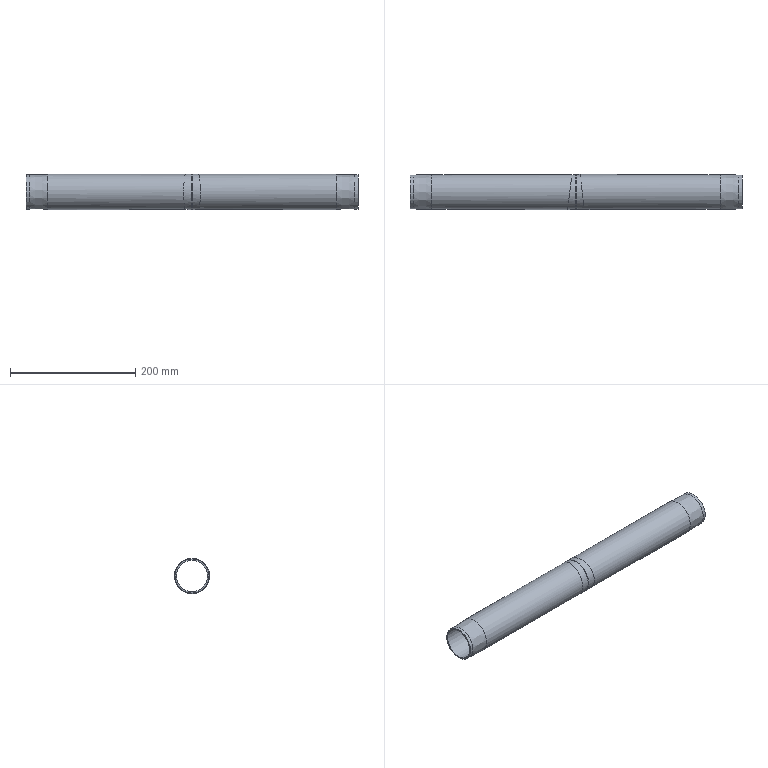Part | STEP file | PN_0012_default | 1 solid | 12 faces | box 530 x 56 x 56 mm | volume 259272 mm3 | cylinder 8 | cone 2 | plane 2 | commonest cylinder face diameters 56 x5 54.429 x2 50 x1
STEP:
#1=CARTESIAN_POINT('',(0.,0.,0.));
#2=DIRECTION('',(0.,0.,1.));
#3=DIRECTION('',(1.,0.,0.));
#4=AXIS2_PLACEMENT_3D('',#1,#2,#3);
#5=CARTESIAN_POINT('',(-0.5,0.,28.));
#6=VERTEX_POINT('',#5);
#7=CARTESIAN_POINT('',(-0.5,0.,0.));
#8=DIRECTION('',(-1.,0.,0.));
#9=DIRECTION('',(0.,0.,1.));
#10=AXIS2_PLACEMENT_3D('',#7,#8,#9);
#11=CIRCLE('',#10,28.);
#12=CARTESIAN_POINT('',(-290.929,0.,0.));
#13=DIRECTION('',(-1.,0.,0.));
#14=DIRECTION('',(0.,0.,1.));
#15=AXIS2_PLACEMENT_3D('',#12,#13,#14);
#16=CYLINDRICAL_SURFACE('',#15,28.);
#17=CARTESIAN_POINT('',(0.,-290.429));
#18=DIRECTION('',(1.,0.));
#19=VECTOR('',#18,1.);
#20=LINE('',#17,#19);
#21=(GEOMETRIC_REPRESENTATION_CONTEXT(2)PARAMETRIC_REPRESENTATION_CONTEXT()REPRESENTATION_CONTEXT('',''));
#22=DEFINITIONAL_REPRESENTATION('',(#20),#21);
#23=PCURVE('',#16,#22);
#24=CARTESIAN_POINT('',(-290.929,0.,0.));
#25=DIRECTION('',(-1.,0.,0.));
#26=DIRECTION('',(0.,0.,1.));
#27=AXIS2_PLACEMENT_3D('',#24,#25,#26);
#28=CYLINDRICAL_SURFACE('',#27,28.);
#29=CARTESIAN_POINT('',(0.,-290.429));
#30=DIRECTION('',(1.,0.));
#31=VECTOR('',#30,1.);
#32=LINE('',#29,#31);
#33=(GEOMETRIC_REPRESENTATION_CONTEXT(2)PARAMETRIC_REPRESENTATION_CONTEXT()REPRESENTATION_CONTEXT('',''));
#34=DEFINITIONAL_REPRESENTATION('',(#32),#33);
#35=PCURVE('',#28,#34);
#36=SURFACE_CURVE('',#11,(#23,#35),.PCURVE_S1.);
#37=EDGE_CURVE('',#6,#6,#36,.T.);
#38=ORIENTED_EDGE('',*,*,#37,.F.);
#39=CARTESIAN_POINT('',(0.5,0.,28.));
#40=VERTEX_POINT('',#39);
#41=CARTESIAN_POINT('',(0.5,0.,28.));
#42=CARTESIAN_POINT('',(-0.5,0.,28.));
#43=B_SPLINE_CURVE_WITH_KNOTS('',1,(#41,#42),.UNSPECIFIED.,.F.,.F.,(2,2),(-291.429,-290.429),.PIECEWISE_BEZIER_KNOTS.);
#44=CARTESIAN_POINT('',(0.,0.));
#45=DIRECTION('',(0.,1.));
#46=VECTOR('',#45,1.);
#47=LINE('',#44,#46);
#48=(GEOMETRIC_REPRESENTATION_CONTEXT(2)PARAMETRIC_REPRESENTATION_CONTEXT()REPRESENTATION_CONTEXT('',''));
#49=DEFINITIONAL_REPRESENTATION('',(#47),#48);
#50=PCURVE('',#16,#49);
#51=CARTESIAN_POINT('',(6.283,0.));
#52=DIRECTION('',(0.,1.));
#53=VECTOR('',#52,1.);
#54=LINE('',#51,#53);
#55=(GEOMETRIC_REPRESENTATION_CONTEXT(2)PARAMETRIC_REPRESENTATION_CONTEXT()REPRESENTATION_CONTEXT('',''));
#56=DEFINITIONAL_REPRESENTATION('',(#54),#55);
#57=PCURVE('',#16,#56);
#58=SEAM_CURVE('',#43,(#50,#57),.PCURVE_S1.);
#59=EDGE_CURVE('',#40,#6,#58,.T.);
#60=ORIENTED_EDGE('',*,*,#59,.F.);
#61=CARTESIAN_POINT('',(0.5,0.,-28.));
#62=VERTEX_POINT('',#61);
#63=CARTESIAN_POINT('',(0.5,0.,0.));
#64=DIRECTION('',(1.,0.,0.));
#65=DIRECTION('',(0.,0.,-1.));
#66=AXIS2_PLACEMENT_3D('',#63,#64,#65);
#67=CIRCLE('',#66,28.);
#68=CARTESIAN_POINT('',(3.142,-291.429));
#69=DIRECTION('',(-1.,0.));
#70=VECTOR('',#69,1.);
#71=LINE('',#68,#70);
#72=(GEOMETRIC_REPRESENTATION_CONTEXT(2)PARAMETRIC_REPRESENTATION_CONTEXT()REPRESENTATION_CONTEXT('',''));
#73=DEFINITIONAL_REPRESENTATION('',(#71),#72);
#74=PCURVE('',#16,#73);
#75=CARTESIAN_POINT('',(-290.929,0.,0.));
#76=DIRECTION('',(-1.,0.,0.));
#77=DIRECTION('',(0.,0.,1.));
#78=AXIS2_PLACEMENT_3D('',#75,#76,#77);
#79=CYLINDRICAL_SURFACE('',#78,28.);
#80=CARTESIAN_POINT('',(3.142,-291.429));
#81=DIRECTION('',(-1.,0.));
#82=VECTOR('',#81,1.);
#83=LINE('',#80,#82);
#84=(GEOMETRIC_REPRESENTATION_CONTEXT(2)PARAMETRIC_REPRESENTATION_CONTEXT()REPRESENTATION_CONTEXT('',''));
#85=DEFINITIONAL_REPRESENTATION('',(#83),#84);
#86=PCURVE('',#79,#85);
#87=SURFACE_CURVE('',#67,(#74,#86),.PCURVE_S1.);
#88=EDGE_CURVE('',#62,#40,#87,.T.);
#89=ORIENTED_EDGE('',*,*,#88,.F.);
#90=CARTESIAN_POINT('',(0.5,0.,0.));
#91=DIRECTION('',(1.,0.,0.));
#92=DIRECTION('',(0.,0.,-1.));
#93=AXIS2_PLACEMENT_3D('',#90,#91,#92);
#94=CIRCLE('',#93,28.);
#95=CARTESIAN_POINT('',(9.425,-291.429));
#96=DIRECTION('',(-1.,0.));
#97=VECTOR('',#96,1.);
#98=LINE('',#95,#97);
#99=(GEOMETRIC_REPRESENTATION_CONTEXT(2)PARAMETRIC_REPRESENTATION_CONTEXT()REPRESENTATION_CONTEXT('',''));
#100=DEFINITIONAL_REPRESENTATION('',(#98),#99);
#101=PCURVE('',#16,#100);
#102=CARTESIAN_POINT('',(9.425,-291.429));
#103=DIRECTION('',(-1.,0.));
#104=VECTOR('',#103,1.);
#105=LINE('',#102,#104);
#106=(GEOMETRIC_REPRESENTATION_CONTEXT(2)PARAMETRIC_REPRESENTATION_CONTEXT()REPRESENTATION_CONTEXT('',''));
#107=DEFINITIONAL_REPRESENTATION('',(#105),#106);
#108=PCURVE('',#79,#107);
#109=SURFACE_CURVE('',#94,(#101,#108),.PCURVE_S1.);
#110=EDGE_CURVE('',#40,#62,#109,.T.);
#111=ORIENTED_EDGE('',*,*,#110,.F.);
#112=ORIENTED_EDGE('',*,*,#59,.T.);
#113=EDGE_LOOP('',(#38,#60,#89,#111,#112));
#114=FACE_BOUND('',#113,.T.);
#115=ADVANCED_FACE('',(#114),#16,.T.);
#116=CARTESIAN_POINT('',(230.,0.,28.));
#117=VERTEX_POINT('',#116);
#118=CARTESIAN_POINT('',(230.,0.,0.));
#119=DIRECTION('',(-1.,0.,0.));
#120=DIRECTION('',(0.,0.,1.));
#121=AXIS2_PLACEMENT_3D('',#118,#119,#120);
#122=CIRCLE('',#121,28.);
#123=CARTESIAN_POINT('',(-290.929,0.,0.));
#124=DIRECTION('',(-1.,0.,0.));
#125=DIRECTION('',(0.,0.,1.));
#126=AXIS2_PLACEMENT_3D('',#123,#124,#125);
#127=CYLINDRICAL_SURFACE('',#126,28.);
#128=CARTESIAN_POINT('',(0.,-520.929));
#129=DIRECTION('',(1.,0.));
#130=VECTOR('',#129,1.);
#131=LINE('',#128,#130);
#132=(GEOMETRIC_REPRESENTATION_CONTEXT(2)PARAMETRIC_REPRESENTATION_CONTEXT()REPRESENTATION_CONTEXT('',''));
#133=DEFINITIONAL_REPRESENTATION('',(#131),#132);
#134=PCURVE('',#127,#133);
#135=CARTESIAN_POINT('',(260.,0.,0.));
#136=DIRECTION('',(-1.,0.,0.));
#137=DIRECTION('',(0.,0.,1.));
#138=AXIS2_PLACEMENT_3D('',#135,#136,#137);
#139=CONICAL_SURFACE('',#138,27.214,0.02618);
#140=CARTESIAN_POINT('',(0.,30.));
#141=DIRECTION('',(1.,0.));
#142=VECTOR('',#141,1.);
#143=LINE('',#140,#142);
#144=(GEOMETRIC_REPRESENTATION_CONTEXT(2)PARAMETRIC_REPRESENTATION_CONTEXT()REPRESENTATION_CONTEXT('',''));
#145=DEFINITIONAL_REPRESENTATION('',(#143),#144);
#146=PCURVE('',#139,#145);
#147=SURFACE_CURVE('',#122,(#134,#146),.PCURVE_S1.);
#148=EDGE_CURVE('',#117,#117,#147,.T.);
#149=ORIENTED_EDGE('',*,*,#148,.T.);
#150=CARTESIAN_POINT('',(9.959,0.,28.));
#151=VERTEX_POINT('',#150);
#152=CARTESIAN_POINT('',(230.,0.,28.));
#153=CARTESIAN_POINT('',(9.959,0.,28.));
#154=B_SPLINE_CURVE_WITH_KNOTS('',1,(#152,#153),.UNSPECIFIED.,.F.,.F.,(2,2),(-520.929,-300.889),.PIECEWISE_BEZIER_KNOTS.);
#155=CARTESIAN_POINT('',(6.283,0.));
#156=DIRECTION('',(0.,1.));
#157=VECTOR('',#156,1.);
#158=LINE('',#155,#157);
#159=(GEOMETRIC_REPRESENTATION_CONTEXT(2)PARAMETRIC_REPRESENTATION_CONTEXT()REPRESENTATION_CONTEXT('',''));
#160=DEFINITIONAL_REPRESENTATION('',(#158),#159);
#161=PCURVE('',#127,#160);
#162=CARTESIAN_POINT('',(0.,0.));
#163=DIRECTION('',(0.,1.));
#164=VECTOR('',#163,1.);
#165=LINE('',#162,#164);
#166=(GEOMETRIC_REPRESENTATION_CONTEXT(2)PARAMETRIC_REPRESENTATION_CONTEXT()REPRESENTATION_CONTEXT('',''));
#167=DEFINITIONAL_REPRESENTATION('',(#165),#166);
#168=PCURVE('',#127,#167);
#169=SEAM_CURVE('',#154,(#161,#168),.PCURVE_S1.);
#170=EDGE_CURVE('',#117,#151,#169,.T.);
#171=ORIENTED_EDGE('',*,*,#170,.T.);
#172=CARTESIAN_POINT('',(6.587,28.,0.));
#173=VERTEX_POINT('',#172);
#174=CARTESIAN_POINT('',(6.587,28.,0.));
#175=CARTESIAN_POINT('',(6.587,28.,-56.));
#176=CARTESIAN_POINT('',(13.332,-28.,-56.));
#177=CARTESIAN_POINT('',(13.332,-28.,0.));
#178=CARTESIAN_POINT('',(13.332,-28.,56.));
#179=CARTESIAN_POINT('',(6.587,28.,56.));
#180=CARTESIAN_POINT('',(6.587,28.,0.));
#181=(BOUNDED_CURVE()B_SPLINE_CURVE(3,(#174,#175,#176,#177,#178,#179,#180),.UNSPECIFIED.,.T.,.F.)B_SPLINE_CURVE_WITH_KNOTS((1,3,3,3,1),(-3.142,0.,3.142,6.283,9.425),.UNSPECIFIED.)CURVE()GEOMETRIC_REPRESENTATION_ITEM()RATIONAL_B_SPLINE_CURVE((1.,0.3333,0.3333,1.,0.3333,0.3333,1.))REPRESENTATION_ITEM(''));
#182=CARTESIAN_POINT('',(1.571,-297.516));
#183=CARTESIAN_POINT('',(1.631,-297.517));
#184=CARTESIAN_POINT('',(1.764,-297.553));
#185=CARTESIAN_POINT('',(2.001,-297.789));
#186=CARTESIAN_POINT('',(2.281,-298.293));
#187=CARTESIAN_POINT('',(2.604,-299.127));
#188=CARTESIAN_POINT('',(2.958,-300.26));
#189=CARTESIAN_POINT('',(3.325,-301.518));
#190=CARTESIAN_POINT('',(3.679,-302.651));
#191=CARTESIAN_POINT('',(4.002,-303.485));
#192=CARTESIAN_POINT('',(4.282,-303.989));
#193=CARTESIAN_POINT('',(4.521,-304.225));
#194=CARTESIAN_POINT('',(4.712,-304.28));
#195=CARTESIAN_POINT('',(4.904,-304.225));
#196=CARTESIAN_POINT('',(5.143,-303.989));
#197=CARTESIAN_POINT('',(5.423,-303.485));
#198=CARTESIAN_POINT('',(5.745,-302.651));
#199=CARTESIAN_POINT('',(6.1,-301.518));
#200=CARTESIAN_POINT('',(6.467,-300.26));
#201=CARTESIAN_POINT('',(6.821,-299.127));
#202=CARTESIAN_POINT('',(7.143,-298.293));
#203=CARTESIAN_POINT('',(7.424,-297.789));
#204=CARTESIAN_POINT('',(7.661,-297.553));
#205=CARTESIAN_POINT('',(7.794,-297.517));
#206=CARTESIAN_POINT('',(7.854,-297.516));
#207=B_SPLINE_CURVE_WITH_KNOTS('',3,(#182,#183,#184,#185,#186,#187,#188,#189,#190,#191,#192,#193,#194,#195,#196,#197,#198,#199,#200,#201,#202,#203,#204,#205,#206),.UNSPECIFIED.,.F.,.F.,(4,1,1,1,1,1,1,1,1,1,1,1,1,1,1,1,1,1,1,1,1,1,4),(0.,0.2856,0.5712,0.8568,1.142,1.428,1.714,1.999,2.285,2.57,2.856,3.142,3.427,3.713,3.998,4.284,4.57,4.855,5.141,5.426,5.712,5.998,6.283),.QUASI_UNIFORM_KNOTS.);
#208=(GEOMETRIC_REPRESENTATION_CONTEXT(2)PARAMETRIC_REPRESENTATION_CONTEXT()REPRESENTATION_CONTEXT('',''));
#209=DEFINITIONAL_REPRESENTATION('',(#207),#208);
#210=PCURVE('',#127,#209);
#211=CARTESIAN_POINT('',(1.571,-297.516));
#212=CARTESIAN_POINT('',(1.616,-297.517));
#213=CARTESIAN_POINT('',(1.713,-297.537));
#214=CARTESIAN_POINT('',(1.88,-297.659));
#215=CARTESIAN_POINT('',(2.07,-297.908));
#216=CARTESIAN_POINT('',(2.284,-298.317));
#217=CARTESIAN_POINT('',(2.522,-298.91));
#218=CARTESIAN_POINT('',(2.78,-299.681));
#219=CARTESIAN_POINT('',(3.05,-300.577));
#220=CARTESIAN_POINT('',(3.324,-301.508));
#221=CARTESIAN_POINT('',(3.591,-302.371));
#222=CARTESIAN_POINT('',(3.843,-303.086));
#223=CARTESIAN_POINT('',(4.073,-303.617));
#224=CARTESIAN_POINT('',(4.279,-303.969));
#225=CARTESIAN_POINT('',(4.461,-304.171));
#226=CARTESIAN_POINT('',(4.622,-304.259));
#227=CARTESIAN_POINT('',(4.756,-304.269));
#228=CARTESIAN_POINT('',(4.908,-304.212));
#229=CARTESIAN_POINT('',(5.082,-304.051));
#230=CARTESIAN_POINT('',(5.28,-303.753));
#231=CARTESIAN_POINT('',(5.503,-303.283));
#232=CARTESIAN_POINT('',(5.748,-302.629));
#233=CARTESIAN_POINT('',(6.011,-301.807));
#234=CARTESIAN_POINT('',(6.192,-301.198));
#235=CARTESIAN_POINT('',(6.283,-300.889));
#236=B_SPLINE_CURVE_WITH_KNOTS('',3,(#211,#212,#213,#214,#215,#216,#217,#218,#219,#220,#221,#222,#223,#224,#225,#226,#227,#228,#229,#230,#231,#232,#233,#234,#235),.UNSPECIFIED.,.F.,.F.,(4,1,1,1,1,1,1,1,1,1,1,1,1,1,1,1,1,1,1,1,1,1,4),(0.,0.2142,0.4284,0.6426,0.8568,1.071,1.285,1.499,1.714,1.928,2.142,2.356,2.57,2.785,2.999,3.213,3.427,3.641,3.856,4.07,4.284,4.498,4.712),.QUASI_UNIFORM_KNOTS.);
#237=(GEOMETRIC_REPRESENTATION_CONTEXT(2)PARAMETRIC_REPRESENTATION_CONTEXT()REPRESENTATION_CONTEXT('',''));
#238=DEFINITIONAL_REPRESENTATION('',(#236),#237);
#239=PCURVE('',#79,#238);
#240=SURFACE_CURVE('',#181,(#210,#239),.PCURVE_S1.);
#241=EDGE_CURVE('',#173,#151,#240,.T.);
#242=ORIENTED_EDGE('',*,*,#241,.F.);
#243=CARTESIAN_POINT('',(6.587,28.,0.));
#244=CARTESIAN_POINT('',(6.587,28.,-56.));
#245=CARTESIAN_POINT('',(13.332,-28.,-56.));
#246=CARTESIAN_POINT('',(13.332,-28.,0.));
#247=CARTESIAN_POINT('',(13.332,-28.,56.));
#248=CARTESIAN_POINT('',(6.587,28.,56.));
#249=CARTESIAN_POINT('',(6.587,28.,0.));
#250=(BOUNDED_CURVE()B_SPLINE_CURVE(3,(#243,#244,#245,#246,#247,#248,#249),.UNSPECIFIED.,.T.,.F.)B_SPLINE_CURVE_WITH_KNOTS((1,3,3,3,1),(-3.142,0.,3.142,6.283,9.425),.UNSPECIFIED.)CURVE()GEOMETRIC_REPRESENTATION_ITEM()RATIONAL_B_SPLINE_CURVE((1.,0.3333,0.3333,1.,0.3333,0.3333,1.))REPRESENTATION_ITEM(''));
#251=CARTESIAN_POINT('',(-4.712,-297.516));
#252=CARTESIAN_POINT('',(-4.652,-297.517));
#253=CARTESIAN_POINT('',(-4.519,-297.553));
#254=CARTESIAN_POINT('',(-4.282,-297.789));
#255=CARTESIAN_POINT('',(-4.002,-298.293));
#256=CARTESIAN_POINT('',(-3.679,-299.127));
#257=CARTESIAN_POINT('',(-3.325,-300.26));
#258=CARTESIAN_POINT('',(-2.958,-301.518));
#259=CARTESIAN_POINT('',(-2.604,-302.651));
#260=CARTESIAN_POINT('',(-2.281,-303.485));
#261=CARTESIAN_POINT('',(-2.001,-303.989));
#262=CARTESIAN_POINT('',(-1.762,-304.225));
#263=CARTESIAN_POINT('',(-1.571,-304.28));
#264=CARTESIAN_POINT('',(-1.379,-304.225));
#265=CARTESIAN_POINT('',(-1.14,-303.989));
#266=CARTESIAN_POINT('',(-0.8604,-303.485));
#267=CARTESIAN_POINT('',(-0.5378,-302.651));
#268=CARTESIAN_POINT('',(-0.1834,-301.518));
#269=CARTESIAN_POINT('',(0.1834,-300.26));
#270=CARTESIAN_POINT('',(0.5379,-299.127));
#271=CARTESIAN_POINT('',(0.8603,-298.293));
#272=CARTESIAN_POINT('',(1.141,-297.789));
#273=CARTESIAN_POINT('',(1.378,-297.553));
#274=CARTESIAN_POINT('',(1.51,-297.517));
#275=CARTESIAN_POINT('',(1.571,-297.516));
#276=B_SPLINE_CURVE_WITH_KNOTS('',3,(#251,#252,#253,#254,#255,#256,#257,#258,#259,#260,#261,#262,#263,#264,#265,#266,#267,#268,#269,#270,#271,#272,#273,#274,#275),.UNSPECIFIED.,.F.,.F.,(4,1,1,1,1,1,1,1,1,1,1,1,1,1,1,1,1,1,1,1,1,1,4),(0.,0.2856,0.5712,0.8568,1.142,1.428,1.714,1.999,2.285,2.57,2.856,3.142,3.427,3.713,3.998,4.284,4.57,4.855,5.141,5.426,5.712,5.998,6.283),.QUASI_UNIFORM_KNOTS.);
#277=(GEOMETRIC_REPRESENTATION_CONTEXT(2)PARAMETRIC_REPRESENTATION_CONTEXT()REPRESENTATION_CONTEXT('',''));
#278=DEFINITIONAL_REPRESENTATION('',(#276),#277);
#279=PCURVE('',#127,#278);
#280=CARTESIAN_POINT('',(0.000002229,-300.889));
#281=CARTESIAN_POINT('',(0.03031,-300.787));
#282=CARTESIAN_POINT('',(0.09091,-300.582));
#283=CARTESIAN_POINT('',(0.1814,-300.279));
#284=CARTESIAN_POINT('',(0.2712,-299.984));
#285=CARTESIAN_POINT('',(0.3599,-299.699));
#286=CARTESIAN_POINT('',(0.4472,-299.428));
#287=CARTESIAN_POINT('',(0.5328,-299.174));
#288=CARTESIAN_POINT('',(0.6165,-298.937));
#289=CARTESIAN_POINT('',(0.6979,-298.719));
#290=CARTESIAN_POINT('',(0.7771,-298.522));
#291=CARTESIAN_POINT('',(0.8537,-298.344));
#292=CARTESIAN_POINT('',(0.9277,-298.187));
#293=CARTESIAN_POINT('',(0.9991,-298.05));
#294=CARTESIAN_POINT('',(1.068,-297.932));
#295=CARTESIAN_POINT('',(1.134,-297.831));
#296=CARTESIAN_POINT('',(1.197,-297.747));
#297=CARTESIAN_POINT('',(1.258,-297.678));
#298=CARTESIAN_POINT('',(1.316,-297.623));
#299=CARTESIAN_POINT('',(1.372,-297.581));
#300=CARTESIAN_POINT('',(1.425,-297.55));
#301=CARTESIAN_POINT('',(1.476,-297.53));
#302=CARTESIAN_POINT('',(1.525,-297.519));
#303=CARTESIAN_POINT('',(1.556,-297.516));
#304=CARTESIAN_POINT('',(1.571,-297.516));
#305=B_SPLINE_CURVE_WITH_KNOTS('',3,(#280,#281,#282,#283,#284,#285,#286,#287,#288,#289,#290,#291,#292,#293,#294,#295,#296,#297,#298,#299,#300,#301,#302,#303,#304),.UNSPECIFIED.,.F.,.F.,(4,1,1,1,1,1,1,1,1,1,1,1,1,1,1,1,1,1,1,1,1,1,4),(4.712,4.784,4.855,4.927,4.998,5.069,5.141,5.212,5.284,5.355,5.426,5.498,5.569,5.641,5.712,5.783,5.855,5.926,5.998,6.069,6.14,6.212,6.283),.QUASI_UNIFORM_KNOTS.);
#306=(GEOMETRIC_REPRESENTATION_CONTEXT(2)PARAMETRIC_REPRESENTATION_CONTEXT()REPRESENTATION_CONTEXT('',''));
#307=DEFINITIONAL_REPRESENTATION('',(#305),#306);
#308=PCURVE('',#79,#307);
#309=SURFACE_CURVE('',#250,(#279,#308),.PCURVE_S1.);
#310=EDGE_CURVE('',#151,#173,#309,.T.);
#311=ORIENTED_EDGE('',*,*,#310,.F.);
#312=ORIENTED_EDGE('',*,*,#170,.F.);
#313=EDGE_LOOP('',(#149,#171,#242,#311,#312));
#314=FACE_BOUND('',#313,.T.);
#315=ADVANCED_FACE('',(#314),#127,.T.);
#316=CARTESIAN_POINT('',(-230.,0.,28.));
#317=VERTEX_POINT('',#316);
#318=CARTESIAN_POINT('',(-230.,0.,0.));
#319=DIRECTION('',(-1.,0.,0.));
#320=DIRECTION('',(0.,0.,1.));
#321=AXIS2_PLACEMENT_3D('',#318,#319,#320);
#322=CIRCLE('',#321,28.);
#323=CARTESIAN_POINT('',(-290.929,0.,0.));
#324=DIRECTION('',(-1.,0.,0.));
#325=DIRECTION('',(0.,0.,1.));
#326=AXIS2_PLACEMENT_3D('',#323,#324,#325);
#327=CYLINDRICAL_SURFACE('',#326,28.);
#328=CARTESIAN_POINT('',(0.,-60.929));
#329=DIRECTION('',(1.,0.));
#330=VECTOR('',#329,1.);
#331=LINE('',#328,#330);
#332=(GEOMETRIC_REPRESENTATION_CONTEXT(2)PARAMETRIC_REPRESENTATION_CONTEXT()REPRESENTATION_CONTEXT('',''));
#333=DEFINITIONAL_REPRESENTATION('',(#331),#332);
#334=PCURVE('',#327,#333);
#335=CARTESIAN_POINT('',(-230.,0.,0.));
#336=DIRECTION('',(1.,0.,0.));
#337=DIRECTION('',(0.,0.,-1.));
#338=AXIS2_PLACEMENT_3D('',#335,#336,#337);
#339=CONICAL_SURFACE('',#338,28.,0.02618);
#340=CARTESIAN_POINT('',(9.425,0.));
#341=DIRECTION('',(-1.,0.));
#342=VECTOR('',#341,1.);
#343=LINE('',#340,#342);
#344=(GEOMETRIC_REPRESENTATION_CONTEXT(2)PARAMETRIC_REPRESENTATION_CONTEXT()REPRESENTATION_CONTEXT('',''));
#345=DEFINITIONAL_REPRESENTATION('',(#343),#344);
#346=PCURVE('',#339,#345);
#347=SURFACE_CURVE('',#322,(#334,#346),.PCURVE_S1.);
#348=EDGE_CURVE('',#317,#317,#347,.T.);
#349=ORIENTED_EDGE('',*,*,#348,.F.);
#350=CARTESIAN_POINT('',(-9.959,0.,28.));
#351=VERTEX_POINT('',#350);
#352=CARTESIAN_POINT('',(-9.959,0.,28.));
#353=CARTESIAN_POINT('',(-230.,0.,28.));
#354=B_SPLINE_CURVE_WITH_KNOTS('',1,(#352,#353),.UNSPECIFIED.,.F.,.F.,(2,2),(-280.97,-60.929),.PIECEWISE_BEZIER_KNOTS.);
#355=CARTESIAN_POINT('',(0.,0.));
#356=DIRECTION('',(0.,1.));
#357=VECTOR('',#356,1.);
#358=LINE('',#355,#357);
#359=(GEOMETRIC_REPRESENTATION_CONTEXT(2)PARAMETRIC_REPRESENTATION_CONTEXT()REPRESENTATION_CONTEXT('',''));
#360=DEFINITIONAL_REPRESENTATION('',(#358),#359);
#361=PCURVE('',#327,#360);
#362=CARTESIAN_POINT('',(6.283,0.));
#363=DIRECTION('',(0.,1.));
#364=VECTOR('',#363,1.);
#365=LINE('',#362,#364);
#366=(GEOMETRIC_REPRESENTATION_CONTEXT(2)PARAMETRIC_REPRESENTATION_CONTEXT()REPRESENTATION_CONTEXT('',''));
#367=DEFINITIONAL_REPRESENTATION('',(#365),#366);
#368=PCURVE('',#327,#367);
#369=SEAM_CURVE('',#354,(#361,#368),.PCURVE_S1.);
#370=EDGE_CURVE('',#351,#317,#369,.T.);
#371=ORIENTED_EDGE('',*,*,#370,.F.);
#372=CARTESIAN_POINT('',(-13.332,-28.,0.));
#373=VERTEX_POINT('',#372);
#374=CARTESIAN_POINT('',(-13.332,-28.,0.));
#375=CARTESIAN_POINT('',(-13.332,-28.,-56.));
#376=CARTESIAN_POINT('',(-6.587,28.,-56.));
#377=CARTESIAN_POINT('',(-6.587,28.,0.));
#378=CARTESIAN_POINT('',(-6.587,28.,56.));
#379=CARTESIAN_POINT('',(-13.332,-28.,56.));
#380=CARTESIAN_POINT('',(-13.332,-28.,0.));
#381=(BOUNDED_CURVE()B_SPLINE_CURVE(3,(#374,#375,#376,#377,#378,#379,#380),.UNSPECIFIED.,.T.,.F.)B_SPLINE_CURVE_WITH_KNOTS((1,3,3,3,1),(-3.142,0.,3.142,6.283,9.425),.UNSPECIFIED.)CURVE()GEOMETRIC_REPRESENTATION_ITEM()RATIONAL_B_SPLINE_CURVE((1.,0.3333,0.3333,1.,0.3333,0.3333,1.))REPRESENTATION_ITEM(''));
#382=CARTESIAN_POINT('',(4.712,-277.597));
#383=CARTESIAN_POINT('',(4.652,-277.598));
#384=CARTESIAN_POINT('',(4.519,-277.634));
#385=CARTESIAN_POINT('',(4.282,-277.87));
#386=CARTESIAN_POINT('',(4.002,-278.374));
#387=CARTESIAN_POINT('',(3.679,-279.208));
#388=CARTESIAN_POINT('',(3.325,-280.341));
#389=CARTESIAN_POINT('',(2.958,-281.599));
#390=CARTESIAN_POINT('',(2.604,-282.732));
#391=CARTESIAN_POINT('',(2.281,-283.566));
#392=CARTESIAN_POINT('',(2.001,-284.07));
#393=CARTESIAN_POINT('',(1.762,-284.306));
#394=CARTESIAN_POINT('',(1.571,-284.361));
#395=CARTESIAN_POINT('',(1.379,-284.306));
#396=CARTESIAN_POINT('',(1.14,-284.07));
#397=CARTESIAN_POINT('',(0.8604,-283.566));
#398=CARTESIAN_POINT('',(0.5378,-282.732));
#399=CARTESIAN_POINT('',(0.1834,-281.599));
#400=CARTESIAN_POINT('',(-0.1834,-280.341));
#401=CARTESIAN_POINT('',(-0.5379,-279.208));
#402=CARTESIAN_POINT('',(-0.8603,-278.374));
#403=CARTESIAN_POINT('',(-1.141,-277.87));
#404=CARTESIAN_POINT('',(-1.378,-277.634));
#405=CARTESIAN_POINT('',(-1.51,-277.598));
#406=CARTESIAN_POINT('',(-1.571,-277.597));
#407=B_SPLINE_CURVE_WITH_KNOTS('',3,(#382,#383,#384,#385,#386,#387,#388,#389,#390,#391,#392,#393,#394,#395,#396,#397,#398,#399,#400,#401,#402,#403,#404,#405,#406),.UNSPECIFIED.,.F.,.F.,(4,1,1,1,1,1,1,1,1,1,1,1,1,1,1,1,1,1,1,1,1,1,4),(0.,0.2856,0.5712,0.8568,1.142,1.428,1.714,1.999,2.285,2.57,2.856,3.142,3.427,3.713,3.998,4.284,4.57,4.855,5.141,5.426,5.712,5.998,6.283),.QUASI_UNIFORM_KNOTS.);
#408=(GEOMETRIC_REPRESENTATION_CONTEXT(2)PARAMETRIC_REPRESENTATION_CONTEXT()REPRESENTATION_CONTEXT('',''));
#409=DEFINITIONAL_REPRESENTATION('',(#407),#408);
#410=PCURVE('',#327,#409);
#411=CARTESIAN_POINT('',(4.712,-277.597));
#412=CARTESIAN_POINT('',(4.667,-277.598));
#413=CARTESIAN_POINT('',(4.57,-277.618));
#414=CARTESIAN_POINT('',(4.403,-277.74));
#415=CARTESIAN_POINT('',(4.213,-277.989));
#416=CARTESIAN_POINT('',(3.999,-278.398));
#417=CARTESIAN_POINT('',(3.761,-278.992));
#418=CARTESIAN_POINT('',(3.503,-279.762));
#419=CARTESIAN_POINT('',(3.233,-280.658));
#420=CARTESIAN_POINT('',(2.959,-281.589));
#421=CARTESIAN_POINT('',(2.692,-282.452));
#422=CARTESIAN_POINT('',(2.44,-283.167));
#423=CARTESIAN_POINT('',(2.21,-283.698));
#424=CARTESIAN_POINT('',(2.004,-284.05));
#425=CARTESIAN_POINT('',(1.822,-284.253));
#426=CARTESIAN_POINT('',(1.662,-284.34));
#427=CARTESIAN_POINT('',(1.527,-284.35));
#428=CARTESIAN_POINT('',(1.375,-284.293));
#429=CARTESIAN_POINT('',(1.201,-284.132));
#430=CARTESIAN_POINT('',(1.003,-283.834));
#431=CARTESIAN_POINT('',(0.7804,-283.365));
#432=CARTESIAN_POINT('',(0.5355,-282.71));
#433=CARTESIAN_POINT('',(0.2726,-281.888));
#434=CARTESIAN_POINT('',(0.09109,-281.279));
#435=CARTESIAN_POINT('',(-0.000002229,-280.97));
#436=B_SPLINE_CURVE_WITH_KNOTS('',3,(#411,#412,#413,#414,#415,#416,#417,#418,#419,#420,#421,#422,#423,#424,#425,#426,#427,#428,#429,#430,#431,#432,#433,#434,#435),.UNSPECIFIED.,.F.,.F.,(4,1,1,1,1,1,1,1,1,1,1,1,1,1,1,1,1,1,1,1,1,1,4),(0.,0.2142,0.4284,0.6426,0.8568,1.071,1.285,1.499,1.714,1.928,2.142,2.356,2.57,2.785,2.999,3.213,3.427,3.641,3.856,4.07,4.284,4.498,4.712),.QUASI_UNIFORM_KNOTS.);
#437=(GEOMETRIC_REPRESENTATION_CONTEXT(2)PARAMETRIC_REPRESENTATION_CONTEXT()REPRESENTATION_CONTEXT('',''));
#438=DEFINITIONAL_REPRESENTATION('',(#436),#437);
#439=PCURVE('',#28,#438);
#440=SURFACE_CURVE('',#381,(#410,#439),.PCURVE_S1.);
#441=EDGE_CURVE('',#373,#351,#440,.T.);
#442=ORIENTED_EDGE('',*,*,#441,.F.);
#443=CARTESIAN_POINT('',(-13.332,-28.,0.));
#444=CARTESIAN_POINT('',(-13.332,-28.,-56.));
#445=CARTESIAN_POINT('',(-6.587,28.,-56.));
#446=CARTESIAN_POINT('',(-6.587,28.,0.));
#447=CARTESIAN_POINT('',(-6.587,28.,56.));
#448=CARTESIAN_POINT('',(-13.332,-28.,56.));
#449=CARTESIAN_POINT('',(-13.332,-28.,0.));
#450=(BOUNDED_CURVE()B_SPLINE_CURVE(3,(#443,#444,#445,#446,#447,#448,#449),.UNSPECIFIED.,.T.,.F.)B_SPLINE_CURVE_WITH_KNOTS((1,3,3,3,1),(-3.142,0.,3.142,6.283,9.425),.UNSPECIFIED.)CURVE()GEOMETRIC_REPRESENTATION_ITEM()RATIONAL_B_SPLINE_CURVE((1.,0.3333,0.3333,1.,0.3333,0.3333,1.))REPRESENTATION_ITEM(''));
#451=CARTESIAN_POINT('',(10.996,-277.597));
#452=CARTESIAN_POINT('',(10.935,-277.598));
#453=CARTESIAN_POINT('',(10.803,-277.634));
#454=CARTESIAN_POINT('',(10.565,-277.87));
#455=CARTESIAN_POINT('',(10.285,-278.374));
#456=CARTESIAN_POINT('',(9.963,-279.208));
#457=CARTESIAN_POINT('',(9.608,-280.341));
#458=CARTESIAN_POINT('',(9.241,-281.599));
#459=CARTESIAN_POINT('',(8.887,-282.732));
#460=CARTESIAN_POINT('',(8.564,-283.566));
#461=CARTESIAN_POINT('',(8.285,-284.07));
#462=CARTESIAN_POINT('',(8.045,-284.306));
#463=CARTESIAN_POINT('',(7.854,-284.361));
#464=CARTESIAN_POINT('',(7.663,-284.306));
#465=CARTESIAN_POINT('',(7.423,-284.07));
#466=CARTESIAN_POINT('',(7.144,-283.566));
#467=CARTESIAN_POINT('',(6.821,-282.732));
#468=CARTESIAN_POINT('',(6.467,-281.599));
#469=CARTESIAN_POINT('',(6.1,-280.341));
#470=CARTESIAN_POINT('',(5.745,-279.208));
#471=CARTESIAN_POINT('',(5.423,-278.374));
#472=CARTESIAN_POINT('',(5.143,-277.87));
#473=CARTESIAN_POINT('',(4.905,-277.634));
#474=CARTESIAN_POINT('',(4.773,-277.598));
#475=CARTESIAN_POINT('',(4.712,-277.597));
#476=B_SPLINE_CURVE_WITH_KNOTS('',3,(#451,#452,#453,#454,#455,#456,#457,#458,#459,#460,#461,#462,#463,#464,#465,#466,#467,#468,#469,#470,#471,#472,#473,#474,#475),.UNSPECIFIED.,.F.,.F.,(4,1,1,1,1,1,1,1,1,1,1,1,1,1,1,1,1,1,1,1,1,1,4),(0.,0.2856,0.5712,0.8568,1.142,1.428,1.714,1.999,2.285,2.57,2.856,3.142,3.427,3.713,3.998,4.284,4.57,4.855,5.141,5.426,5.712,5.998,6.283),.QUASI_UNIFORM_KNOTS.);
#477=(GEOMETRIC_REPRESENTATION_CONTEXT(2)PARAMETRIC_REPRESENTATION_CONTEXT()REPRESENTATION_CONTEXT('',''));
#478=DEFINITIONAL_REPRESENTATION('',(#476),#477);
#479=PCURVE('',#327,#478);
#480=CARTESIAN_POINT('',(6.283,-280.97));
#481=CARTESIAN_POINT('',(6.253,-280.868));
#482=CARTESIAN_POINT('',(6.192,-280.663));
#483=CARTESIAN_POINT('',(6.102,-280.36));
#484=CARTESIAN_POINT('',(6.012,-280.065));
#485=CARTESIAN_POINT('',(5.923,-279.78));
#486=CARTESIAN_POINT('',(5.836,-279.51));
#487=CARTESIAN_POINT('',(5.75,-279.255));
#488=CARTESIAN_POINT('',(5.667,-279.018));
#489=CARTESIAN_POINT('',(5.585,-278.8));
#490=CARTESIAN_POINT('',(5.506,-278.603));
#491=CARTESIAN_POINT('',(5.429,-278.426));
#492=CARTESIAN_POINT('',(5.355,-278.269));
#493=CARTESIAN_POINT('',(5.284,-278.131));
#494=CARTESIAN_POINT('',(5.215,-278.013));
#495=CARTESIAN_POINT('',(5.149,-277.912));
#496=CARTESIAN_POINT('',(5.086,-277.828));
#497=CARTESIAN_POINT('',(5.025,-277.759));
#498=CARTESIAN_POINT('',(4.967,-277.704));
#499=CARTESIAN_POINT('',(4.911,-277.662));
#500=CARTESIAN_POINT('',(4.858,-277.632));
#501=CARTESIAN_POINT('',(4.807,-277.611));
#502=CARTESIAN_POINT('',(4.759,-277.6));
#503=CARTESIAN_POINT('',(4.728,-277.597));
#504=CARTESIAN_POINT('',(4.712,-277.597));
#505=B_SPLINE_CURVE_WITH_KNOTS('',3,(#480,#481,#482,#483,#484,#485,#486,#487,#488,#489,#490,#491,#492,#493,#494,#495,#496,#497,#498,#499,#500,#501,#502,#503,#504),.UNSPECIFIED.,.F.,.F.,(4,1,1,1,1,1,1,1,1,1,1,1,1,1,1,1,1,1,1,1,1,1,4),(4.712,4.784,4.855,4.927,4.998,5.069,5.141,5.212,5.284,5.355,5.426,5.498,5.569,5.641,5.712,5.783,5.855,5.926,5.998,6.069,6.14,6.212,6.283),.QUASI_UNIFORM_KNOTS.);
#506=(GEOMETRIC_REPRESENTATION_CONTEXT(2)PARAMETRIC_REPRESENTATION_CONTEXT()REPRESENTATION_CONTEXT('',''));
#507=DEFINITIONAL_REPRESENTATION('',(#505),#506);
#508=PCURVE('',#28,#507);
#509=SURFACE_CURVE('',#450,(#479,#508),.PCURVE_S1.);
#510=EDGE_CURVE('',#351,#373,#509,.T.);
#511=ORIENTED_EDGE('',*,*,#510,.F.);
#512=ORIENTED_EDGE('',*,*,#370,.T.);
#513=EDGE_LOOP('',(#349,#371,#442,#511,#512));
#514=FACE_BOUND('',#513,.T.);
#515=ADVANCED_FACE('',(#514),#327,.T.);
#516=ORIENTED_EDGE('',*,*,#88,.T.);
#517=CARTESIAN_POINT('',(9.959,0.,28.));
#518=CARTESIAN_POINT('',(0.5,0.,28.));
#519=B_SPLINE_CURVE_WITH_KNOTS('',1,(#517,#518),.UNSPECIFIED.,.F.,.F.,(2,2),(-300.889,-291.429),.PIECEWISE_BEZIER_KNOTS.);
#520=CARTESIAN_POINT('',(0.,0.));
#521=DIRECTION('',(0.,1.));
#522=VECTOR('',#521,1.);
#523=LINE('',#520,#522);
#524=(GEOMETRIC_REPRESENTATION_CONTEXT(2)PARAMETRIC_REPRESENTATION_CONTEXT()REPRESENTATION_CONTEXT('',''));
#525=DEFINITIONAL_REPRESENTATION('',(#523),#524);
#526=PCURVE('',#79,#525);
#527=CARTESIAN_POINT('',(6.283,0.));
#528=DIRECTION('',(0.,1.));
#529=VECTOR('',#528,1.);
#530=LINE('',#527,#529);
#531=(GEOMETRIC_REPRESENTATION_CONTEXT(2)PARAMETRIC_REPRESENTATION_CONTEXT()REPRESENTATION_CONTEXT('',''));
#532=DEFINITIONAL_REPRESENTATION('',(#530),#531);
#533=PCURVE('',#79,#532);
#534=SEAM_CURVE('',#519,(#526,#533),.PCURVE_S1.);
#535=EDGE_CURVE('',#151,#40,#534,.T.);
#536=ORIENTED_EDGE('',*,*,#535,.F.);
#537=ORIENTED_EDGE('',*,*,#310,.T.);
#538=ORIENTED_EDGE('',*,*,#241,.T.);
#539=ORIENTED_EDGE('',*,*,#535,.T.);
#540=ORIENTED_EDGE('',*,*,#110,.T.);
#541=EDGE_LOOP('',(#516,#536,#537,#538,#539,#540));
#542=FACE_BOUND('',#541,.T.);
#543=ADVANCED_FACE('',(#542),#79,.T.);
#544=CARTESIAN_POINT('',(-260.,0.,27.214));
#545=VERTEX_POINT('',#544);
#546=CARTESIAN_POINT('',(-260.,0.,0.));
#547=DIRECTION('',(-1.,0.,0.));
#548=DIRECTION('',(0.,0.,1.));
#549=AXIS2_PLACEMENT_3D('',#546,#547,#548);
#550=CIRCLE('',#549,27.214);
#551=CARTESIAN_POINT('',(9.425,-30.));
#552=DIRECTION('',(-1.,0.));
#553=VECTOR('',#552,1.);
#554=LINE('',#551,#553);
#555=(GEOMETRIC_REPRESENTATION_CONTEXT(2)PARAMETRIC_REPRESENTATION_CONTEXT()REPRESENTATION_CONTEXT('',''));
#556=DEFINITIONAL_REPRESENTATION('',(#554),#555);
#557=PCURVE('',#339,#556);
#558=CARTESIAN_POINT('',(-290.929,0.,0.));
#559=DIRECTION('',(-1.,0.,0.));
#560=DIRECTION('',(0.,0.,1.));
#561=AXIS2_PLACEMENT_3D('',#558,#559,#560);
#562=CYLINDRICAL_SURFACE('',#561,27.214);
#563=CARTESIAN_POINT('',(0.,-30.929));
#564=DIRECTION('',(1.,0.));
#565=VECTOR('',#564,1.);
#566=LINE('',#563,#565);
#567=(GEOMETRIC_REPRESENTATION_CONTEXT(2)PARAMETRIC_REPRESENTATION_CONTEXT()REPRESENTATION_CONTEXT('',''));
#568=DEFINITIONAL_REPRESENTATION('',(#566),#567);
#569=PCURVE('',#562,#568);
#570=SURFACE_CURVE('',#550,(#557,#569),.PCURVE_S1.);
#571=EDGE_CURVE('',#545,#545,#570,.T.);
#572=ORIENTED_EDGE('',*,*,#571,.F.);
#573=CARTESIAN_POINT('',(-260.,0.,27.214));
#574=CARTESIAN_POINT('',(-230.,0.,28.));
#575=B_SPLINE_CURVE_WITH_KNOTS('',1,(#573,#574),.UNSPECIFIED.,.F.,.F.,(2,2),(-30.01,0.),.PIECEWISE_BEZIER_KNOTS.);
#576=CARTESIAN_POINT('',(9.425,0.));
#577=DIRECTION('',(0.,1.));
#578=VECTOR('',#577,1.);
#579=LINE('',#576,#578);
#580=(GEOMETRIC_REPRESENTATION_CONTEXT(2)PARAMETRIC_REPRESENTATION_CONTEXT()REPRESENTATION_CONTEXT('',''));
#581=DEFINITIONAL_REPRESENTATION('',(#579),#580);
#582=PCURVE('',#339,#581);
#583=CARTESIAN_POINT('',(3.142,0.));
#584=DIRECTION('',(0.,1.));
#585=VECTOR('',#584,1.);
#586=LINE('',#583,#585);
#587=(GEOMETRIC_REPRESENTATION_CONTEXT(2)PARAMETRIC_REPRESENTATION_CONTEXT()REPRESENTATION_CONTEXT('',''));
#588=DEFINITIONAL_REPRESENTATION('',(#586),#587);
#589=PCURVE('',#339,#588);
#590=SEAM_CURVE('',#575,(#582,#589),.PCURVE_S1.);
#591=EDGE_CURVE('',#545,#317,#590,.T.);
#592=ORIENTED_EDGE('',*,*,#591,.T.);
#593=ORIENTED_EDGE('',*,*,#348,.T.);
#594=ORIENTED_EDGE('',*,*,#591,.F.);
#595=EDGE_LOOP('',(#572,#592,#593,#594));
#596=FACE_BOUND('',#595,.T.);
#597=ADVANCED_FACE('',(#596),#339,.T.);
#598=CARTESIAN_POINT('',(-265.,0.,27.214));
#599=VERTEX_POINT('',#598);
#600=CARTESIAN_POINT('',(-265.,0.,0.));
#601=DIRECTION('',(-1.,0.,0.));
#602=DIRECTION('',(0.,0.,1.));
#603=AXIS2_PLACEMENT_3D('',#600,#601,#602);
#604=CIRCLE('',#603,27.214);
#605=CARTESIAN_POINT('',(0.,-25.929));
#606=DIRECTION('',(1.,0.));
#607=VECTOR('',#606,1.);
#608=LINE('',#605,#607);
#609=(GEOMETRIC_REPRESENTATION_CONTEXT(2)PARAMETRIC_REPRESENTATION_CONTEXT()REPRESENTATION_CONTEXT('',''));
#610=DEFINITIONAL_REPRESENTATION('',(#608),#609);
#611=PCURVE('',#562,#610);
#612=CARTESIAN_POINT('',(-265.,27.214,0.));
#613=DIRECTION('',(1.,0.,0.));
#614=DIRECTION('',(0.,0.,-1.));
#615=AXIS2_PLACEMENT_3D('',#612,#613,#614);
#616=PLANE('',#615);
#617=CARTESIAN_POINT('',(-27.214,-27.214));
#618=CARTESIAN_POINT('',(-27.214,19.922));
#619=CARTESIAN_POINT('',(13.607,-3.646));
#620=CARTESIAN_POINT('',(54.429,-27.214));
#621=CARTESIAN_POINT('',(13.607,-50.783));
#622=CARTESIAN_POINT('',(-27.214,-74.351));
#623=CARTESIAN_POINT('',(-27.214,-27.214));
#624=(BOUNDED_CURVE()B_SPLINE_CURVE(2,(#617,#618,#619,#620,#621,#622,#623),.UNSPECIFIED.,.T.,.F.)B_SPLINE_CURVE_WITH_KNOTS((1,2,2,2,2,1),(-2.094,0.,2.094,4.189,6.283,8.378),.UNSPECIFIED.)CURVE()GEOMETRIC_REPRESENTATION_ITEM()RATIONAL_B_SPLINE_CURVE((1.,0.5,1.,0.5,1.,0.5,1.))REPRESENTATION_ITEM(''));
#625=(GEOMETRIC_REPRESENTATION_CONTEXT(2)PARAMETRIC_REPRESENTATION_CONTEXT()REPRESENTATION_CONTEXT('',''));
#626=DEFINITIONAL_REPRESENTATION('',(#624),#625);
#627=PCURVE('',#616,#626);
#628=SURFACE_CURVE('',#604,(#611,#627),.PCURVE_S1.);
#629=EDGE_CURVE('',#599,#599,#628,.T.);
#630=ORIENTED_EDGE('',*,*,#629,.F.);
#631=CARTESIAN_POINT('',(-260.,0.,27.214));
#632=CARTESIAN_POINT('',(-265.,0.,27.214));
#633=B_SPLINE_CURVE_WITH_KNOTS('',1,(#631,#632),.UNSPECIFIED.,.F.,.F.,(2,2),(-30.929,-25.929),.PIECEWISE_BEZIER_KNOTS.);
#634=CARTESIAN_POINT('',(0.,0.));
#635=DIRECTION('',(0.,1.));
#636=VECTOR('',#635,1.);
#637=LINE('',#634,#636);
#638=(GEOMETRIC_REPRESENTATION_CONTEXT(2)PARAMETRIC_REPRESENTATION_CONTEXT()REPRESENTATION_CONTEXT('',''));
#639=DEFINITIONAL_REPRESENTATION('',(#637),#638);
#640=PCURVE('',#562,#639);
#641=CARTESIAN_POINT('',(6.283,0.));
#642=DIRECTION('',(0.,1.));
#643=VECTOR('',#642,1.);
#644=LINE('',#641,#643);
#645=(GEOMETRIC_REPRESENTATION_CONTEXT(2)PARAMETRIC_REPRESENTATION_CONTEXT()REPRESENTATION_CONTEXT('',''));
#646=DEFINITIONAL_REPRESENTATION('',(#644),#645);
#647=PCURVE('',#562,#646);
#648=SEAM_CURVE('',#633,(#640,#647),.PCURVE_S1.);
#649=EDGE_CURVE('',#545,#599,#648,.T.);
#650=ORIENTED_EDGE('',*,*,#649,.F.);
#651=ORIENTED_EDGE('',*,*,#571,.T.);
#652=ORIENTED_EDGE('',*,*,#649,.T.);
#653=EDGE_LOOP('',(#630,#650,#651,#652));
#654=FACE_BOUND('',#653,.T.);
#655=ADVANCED_FACE('',(#654),#562,.T.);
#656=CARTESIAN_POINT('',(-265.,0.,25.));
#657=VERTEX_POINT('',#656);
#658=CARTESIAN_POINT('',(-265.,0.,0.));
#659=DIRECTION('',(-1.,0.,0.));
#660=DIRECTION('',(0.,0.,1.));
#661=AXIS2_PLACEMENT_3D('',#658,#659,#660);
#662=CIRCLE('',#661,25.);
#663=CARTESIAN_POINT('',(-25.,-27.214));
#664=CARTESIAN_POINT('',(-25.,16.087));
#665=CARTESIAN_POINT('',(12.5,-5.564));
#666=CARTESIAN_POINT('',(50.,-27.214));
#667=CARTESIAN_POINT('',(12.5,-48.865));
#668=CARTESIAN_POINT('',(-25.,-70.516));
#669=CARTESIAN_POINT('',(-25.,-27.214));
#670=(BOUNDED_CURVE()B_SPLINE_CURVE(2,(#663,#664,#665,#666,#667,#668,#669),.UNSPECIFIED.,.T.,.F.)B_SPLINE_CURVE_WITH_KNOTS((1,2,2,2,2,1),(-2.094,0.,2.094,4.189,6.283,8.378),.UNSPECIFIED.)CURVE()GEOMETRIC_REPRESENTATION_ITEM()RATIONAL_B_SPLINE_CURVE((1.,0.5,1.,0.5,1.,0.5,1.))REPRESENTATION_ITEM(''));
#671=(GEOMETRIC_REPRESENTATION_CONTEXT(2)PARAMETRIC_REPRESENTATION_CONTEXT()REPRESENTATION_CONTEXT('',''));
#672=DEFINITIONAL_REPRESENTATION('',(#670),#671);
#673=PCURVE('',#616,#672);
#674=CARTESIAN_POINT('',(-290.929,0.,0.));
#675=DIRECTION('',(-1.,0.,0.));
#676=DIRECTION('',(0.,0.,1.));
#677=AXIS2_PLACEMENT_3D('',#674,#675,#676);
#678=CYLINDRICAL_SURFACE('',#677,25.);
#679=CARTESIAN_POINT('',(0.,-25.929));
#680=DIRECTION('',(1.,0.));
#681=VECTOR('',#680,1.);
#682=LINE('',#679,#681);
#683=(GEOMETRIC_REPRESENTATION_CONTEXT(2)PARAMETRIC_REPRESENTATION_CONTEXT()REPRESENTATION_CONTEXT('',''));
#684=DEFINITIONAL_REPRESENTATION('',(#682),#683);
#685=PCURVE('',#678,#684);
#686=SURFACE_CURVE('',#662,(#673,#685),.PCURVE_S1.);
#687=EDGE_CURVE('',#657,#657,#686,.T.);
#688=ORIENTED_EDGE('',*,*,#687,.F.);
#689=EDGE_LOOP('',(#688));
#690=FACE_BOUND('',#689,.T.);
#691=ORIENTED_EDGE('',*,*,#629,.T.);
#692=EDGE_LOOP('',(#691));
#693=FACE_BOUND('',#692,.T.);
#694=ADVANCED_FACE('',(#690,#693),#616,.F.);
#695=CARTESIAN_POINT('',(265.,0.,25.));
#696=VERTEX_POINT('',#695);
#697=CARTESIAN_POINT('',(265.,0.,0.));
#698=DIRECTION('',(-1.,0.,0.));
#699=DIRECTION('',(0.,0.,1.));
#700=AXIS2_PLACEMENT_3D('',#697,#698,#699);
#701=CIRCLE('',#700,25.);
#702=CARTESIAN_POINT('',(0.,-555.929));
#703=DIRECTION('',(1.,0.));
#704=VECTOR('',#703,1.);
#705=LINE('',#702,#704);
#706=(GEOMETRIC_REPRESENTATION_CONTEXT(2)PARAMETRIC_REPRESENTATION_CONTEXT()REPRESENTATION_CONTEXT('',''));
#707=DEFINITIONAL_REPRESENTATION('',(#705),#706);
#708=PCURVE('',#678,#707);
#709=CARTESIAN_POINT('',(265.,27.214,0.));
#710=DIRECTION('',(-1.,0.,0.));
#711=DIRECTION('',(0.,0.,1.));
#712=AXIS2_PLACEMENT_3D('',#709,#710,#711);
#713=PLANE('',#712);
#714=CARTESIAN_POINT('',(0.,-27.214));
#715=DIRECTION('',(1.,0.));
#716=AXIS2_PLACEMENT_2D('',#714,#715);
#717=CIRCLE('',#716,25.);
#718=(GEOMETRIC_REPRESENTATION_CONTEXT(2)PARAMETRIC_REPRESENTATION_CONTEXT()REPRESENTATION_CONTEXT('',''));
#719=DEFINITIONAL_REPRESENTATION('',(#717),#718);
#720=PCURVE('',#713,#719);
#721=SURFACE_CURVE('',#701,(#708,#720),.PCURVE_S1.);
#722=EDGE_CURVE('',#696,#696,#721,.T.);
#723=ORIENTED_EDGE('',*,*,#722,.T.);
#724=CARTESIAN_POINT('',(265.,0.,25.));
#725=CARTESIAN_POINT('',(-265.,0.,25.));
#726=B_SPLINE_CURVE_WITH_KNOTS('',1,(#724,#725),.UNSPECIFIED.,.F.,.F.,(2,2),(-555.929,-25.929),.PIECEWISE_BEZIER_KNOTS.);
#727=CARTESIAN_POINT('',(6.283,0.));
#728=DIRECTION('',(0.,1.));
#729=VECTOR('',#728,1.);
#730=LINE('',#727,#729);
#731=(GEOMETRIC_REPRESENTATION_CONTEXT(2)PARAMETRIC_REPRESENTATION_CONTEXT()REPRESENTATION_CONTEXT('',''));
#732=DEFINITIONAL_REPRESENTATION('',(#730),#731);
#733=PCURVE('',#678,#732);
#734=CARTESIAN_POINT('',(0.,0.));
#735=DIRECTION('',(0.,1.));
#736=VECTOR('',#735,1.);
#737=LINE('',#734,#736);
#738=(GEOMETRIC_REPRESENTATION_CONTEXT(2)PARAMETRIC_REPRESENTATION_CONTEXT()REPRESENTATION_CONTEXT('',''));
#739=DEFINITIONAL_REPRESENTATION('',(#737),#738);
#740=PCURVE('',#678,#739);
#741=SEAM_CURVE('',#726,(#733,#740),.PCURVE_S1.);
#742=EDGE_CURVE('',#696,#657,#741,.T.);
#743=ORIENTED_EDGE('',*,*,#742,.T.);
#744=ORIENTED_EDGE('',*,*,#687,.F.);
#745=ORIENTED_EDGE('',*,*,#742,.F.);
#746=EDGE_LOOP('',(#723,#743,#744,#745));
#747=FACE_BOUND('',#746,.F.);
#748=ADVANCED_FACE('',(#747),#678,.F.);
#749=CARTESIAN_POINT('',(265.,0.,27.214));
#750=VERTEX_POINT('',#749);
#751=CARTESIAN_POINT('',(265.,0.,0.));
#752=DIRECTION('',(-1.,0.,0.));
#753=DIRECTION('',(0.,0.,1.));
#754=AXIS2_PLACEMENT_3D('',#751,#752,#753);
#755=CIRCLE('',#754,27.214);
#756=CARTESIAN_POINT('',(0.,-27.214));
#757=DIRECTION('',(1.,0.));
#758=AXIS2_PLACEMENT_2D('',#756,#757);
#759=CIRCLE('',#758,27.214);
#760=(GEOMETRIC_REPRESENTATION_CONTEXT(2)PARAMETRIC_REPRESENTATION_CONTEXT()REPRESENTATION_CONTEXT('',''));
#761=DEFINITIONAL_REPRESENTATION('',(#759),#760);
#762=PCURVE('',#713,#761);
#763=CARTESIAN_POINT('',(-290.929,0.,0.));
#764=DIRECTION('',(-1.,0.,0.));
#765=DIRECTION('',(0.,0.,1.));
#766=AXIS2_PLACEMENT_3D('',#763,#764,#765);
#767=CYLINDRICAL_SURFACE('',#766,27.214);
#768=CARTESIAN_POINT('',(0.,-555.929));
#769=DIRECTION('',(1.,0.));
#770=VECTOR('',#769,1.);
#771=LINE('',#768,#770);
#772=(GEOMETRIC_REPRESENTATION_CONTEXT(2)PARAMETRIC_REPRESENTATION_CONTEXT()REPRESENTATION_CONTEXT('',''));
#773=DEFINITIONAL_REPRESENTATION('',(#771),#772);
#774=PCURVE('',#767,#773);
#775=SURFACE_CURVE('',#755,(#762,#774),.PCURVE_S1.);
#776=EDGE_CURVE('',#750,#750,#775,.T.);
#777=ORIENTED_EDGE('',*,*,#776,.F.);
#778=EDGE_LOOP('',(#777));
#779=FACE_BOUND('',#778,.T.);
#780=ORIENTED_EDGE('',*,*,#722,.T.);
#781=EDGE_LOOP('',(#780));
#782=FACE_BOUND('',#781,.T.);
#783=ADVANCED_FACE('',(#779,#782),#713,.F.);
#784=CARTESIAN_POINT('',(260.,0.,27.214));
#785=VERTEX_POINT('',#784);
#786=CARTESIAN_POINT('',(260.,0.,0.));
#787=DIRECTION('',(-1.,0.,0.));
#788=DIRECTION('',(0.,0.,1.));
#789=AXIS2_PLACEMENT_3D('',#786,#787,#788);
#790=CIRCLE('',#789,27.214);
#791=CARTESIAN_POINT('',(0.,-550.929));
#792=DIRECTION('',(1.,0.));
#793=VECTOR('',#792,1.);
#794=LINE('',#791,#793);
#795=(GEOMETRIC_REPRESENTATION_CONTEXT(2)PARAMETRIC_REPRESENTATION_CONTEXT()REPRESENTATION_CONTEXT('',''));
#796=DEFINITIONAL_REPRESENTATION('',(#794),#795);
#797=PCURVE('',#767,#796);
#798=CARTESIAN_POINT('',(0.,0.));
#799=DIRECTION('',(1.,0.));
#800=VECTOR('',#799,1.);
#801=LINE('',#798,#800);
#802=(GEOMETRIC_REPRESENTATION_CONTEXT(2)PARAMETRIC_REPRESENTATION_CONTEXT()REPRESENTATION_CONTEXT('',''));
#803=DEFINITIONAL_REPRESENTATION('',(#801),#802);
#804=PCURVE('',#139,#803);
#805=SURFACE_CURVE('',#790,(#797,#804),.PCURVE_S1.);
#806=EDGE_CURVE('',#785,#785,#805,.T.);
#807=ORIENTED_EDGE('',*,*,#806,.F.);
#808=CARTESIAN_POINT('',(265.,0.,27.214));
#809=CARTESIAN_POINT('',(260.,0.,27.214));
#810=B_SPLINE_CURVE_WITH_KNOTS('',1,(#808,#809),.UNSPECIFIED.,.F.,.F.,(2,2),(-555.929,-550.929),.PIECEWISE_BEZIER_KNOTS.);
#811=CARTESIAN_POINT('',(0.,0.));
#812=DIRECTION('',(0.,1.));
#813=VECTOR('',#812,1.);
#814=LINE('',#811,#813);
#815=(GEOMETRIC_REPRESENTATION_CONTEXT(2)PARAMETRIC_REPRESENTATION_CONTEXT()REPRESENTATION_CONTEXT('',''));
#816=DEFINITIONAL_REPRESENTATION('',(#814),#815);
#817=PCURVE('',#767,#816);
#818=CARTESIAN_POINT('',(6.283,0.));
#819=DIRECTION('',(0.,1.));
#820=VECTOR('',#819,1.);
#821=LINE('',#818,#820);
#822=(GEOMETRIC_REPRESENTATION_CONTEXT(2)PARAMETRIC_REPRESENTATION_CONTEXT()REPRESENTATION_CONTEXT('',''));
#823=DEFINITIONAL_REPRESENTATION('',(#821),#822);
#824=PCURVE('',#767,#823);
#825=SEAM_CURVE('',#810,(#817,#824),.PCURVE_S1.);
#826=EDGE_CURVE('',#750,#785,#825,.T.);
#827=ORIENTED_EDGE('',*,*,#826,.F.);
#828=ORIENTED_EDGE('',*,*,#776,.T.);
#829=ORIENTED_EDGE('',*,*,#826,.T.);
#830=EDGE_LOOP('',(#807,#827,#828,#829));
#831=FACE_BOUND('',#830,.T.);
#832=ADVANCED_FACE('',(#831),#767,.T.);
#833=ORIENTED_EDGE('',*,*,#148,.F.);
#834=CARTESIAN_POINT('',(260.,0.,27.214));
#835=CARTESIAN_POINT('',(230.,0.,28.));
#836=B_SPLINE_CURVE_WITH_KNOTS('',1,(#834,#835),.UNSPECIFIED.,.F.,.F.,(2,2),(0.,30.01),.PIECEWISE_BEZIER_KNOTS.);
#837=CARTESIAN_POINT('',(0.,0.));
#838=DIRECTION('',(0.,1.));
#839=VECTOR('',#838,1.);
#840=LINE('',#837,#839);
#841=(GEOMETRIC_REPRESENTATION_CONTEXT(2)PARAMETRIC_REPRESENTATION_CONTEXT()REPRESENTATION_CONTEXT('',''));
#842=DEFINITIONAL_REPRESENTATION('',(#840),#841);
#843=PCURVE('',#139,#842);
#844=CARTESIAN_POINT('',(6.283,0.));
#845=DIRECTION('',(0.,1.));
#846=VECTOR('',#845,1.);
#847=LINE('',#844,#846);
#848=(GEOMETRIC_REPRESENTATION_CONTEXT(2)PARAMETRIC_REPRESENTATION_CONTEXT()REPRESENTATION_CONTEXT('',''));
#849=DEFINITIONAL_REPRESENTATION('',(#847),#848);
#850=PCURVE('',#139,#849);
#851=SEAM_CURVE('',#836,(#843,#850),.PCURVE_S1.);
#852=EDGE_CURVE('',#785,#117,#851,.T.);
#853=ORIENTED_EDGE('',*,*,#852,.F.);
#854=ORIENTED_EDGE('',*,*,#806,.T.);
#855=ORIENTED_EDGE('',*,*,#852,.T.);
#856=EDGE_LOOP('',(#833,#853,#854,#855));
#857=FACE_BOUND('',#856,.T.);
#858=ADVANCED_FACE('',(#857),#139,.T.);
#859=ORIENTED_EDGE('',*,*,#441,.T.);
#860=CARTESIAN_POINT('',(-0.5,0.,28.));
#861=CARTESIAN_POINT('',(-9.959,0.,28.));
#862=B_SPLINE_CURVE_WITH_KNOTS('',1,(#860,#861),.UNSPECIFIED.,.F.,.F.,(2,2),(-290.429,-280.97),.PIECEWISE_BEZIER_KNOTS.);
#863=CARTESIAN_POINT('',(0.,0.));
#864=DIRECTION('',(0.,1.));
#865=VECTOR('',#864,1.);
#866=LINE('',#863,#865);
#867=(GEOMETRIC_REPRESENTATION_CONTEXT(2)PARAMETRIC_REPRESENTATION_CONTEXT()REPRESENTATION_CONTEXT('',''));
#868=DEFINITIONAL_REPRESENTATION('',(#866),#867);
#869=PCURVE('',#28,#868);
#870=CARTESIAN_POINT('',(6.283,0.));
#871=DIRECTION('',(0.,1.));
#872=VECTOR('',#871,1.);
#873=LINE('',#870,#872);
#874=(GEOMETRIC_REPRESENTATION_CONTEXT(2)PARAMETRIC_REPRESENTATION_CONTEXT()REPRESENTATION_CONTEXT('',''));
#875=DEFINITIONAL_REPRESENTATION('',(#873),#874);
#876=PCURVE('',#28,#875);
#877=SEAM_CURVE('',#862,(#869,#876),.PCURVE_S1.);
#878=EDGE_CURVE('',#6,#351,#877,.T.);
#879=ORIENTED_EDGE('',*,*,#878,.F.);
#880=ORIENTED_EDGE('',*,*,#37,.T.);
#881=ORIENTED_EDGE('',*,*,#878,.T.);
#882=ORIENTED_EDGE('',*,*,#510,.T.);
#883=EDGE_LOOP('',(#859,#879,#880,#881,#882));
#884=FACE_BOUND('',#883,.T.);
#885=ADVANCED_FACE('',(#884),#28,.T.);
#886=CLOSED_SHELL('',(#115,#315,#515,#543,#597,#655,#694,#748,#783,#832,#858,#885));
#887=MANIFOLD_SOLID_BREP('',#886);
#888=(LENGTH_UNIT()NAMED_UNIT(*)SI_UNIT(.MILLI.,.METRE.));
#889=UNCERTAINTY_MEASURE_WITH_UNIT(LENGTH_MEASURE(0.01),#888,'','');
#890=(NAMED_UNIT(*)PLANE_ANGLE_UNIT()SI_UNIT($,.RADIAN.));
#891=(NAMED_UNIT(*)SI_UNIT($,.STERADIAN.)SOLID_ANGLE_UNIT());
#892=(GEOMETRIC_REPRESENTATION_CONTEXT(3)GLOBAL_UNCERTAINTY_ASSIGNED_CONTEXT((#889))GLOBAL_UNIT_ASSIGNED_CONTEXT((#888,#890,#891))REPRESENTATION_CONTEXT('',''));
#893=ADVANCED_BREP_SHAPE_REPRESENTATION('',(#4,#887),#892);